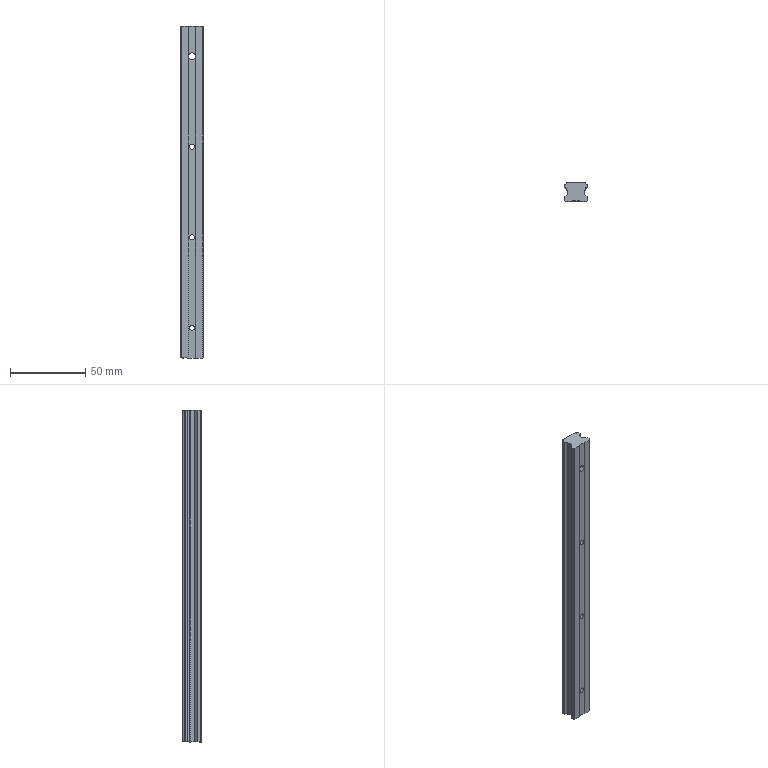Part | SolidWorks | features BaseBody 1, HoleWzd 1, MoveFace 1 | 1 solid | 59 faces | box 15 x 12.5 x 220 mm | volume 34973 mm3 | cylinder 34 | plane 25 | commonest cylinder face diameters 0.6 x11 3.5 x6 6 x6 3 x5 1 x2 4.5 x2